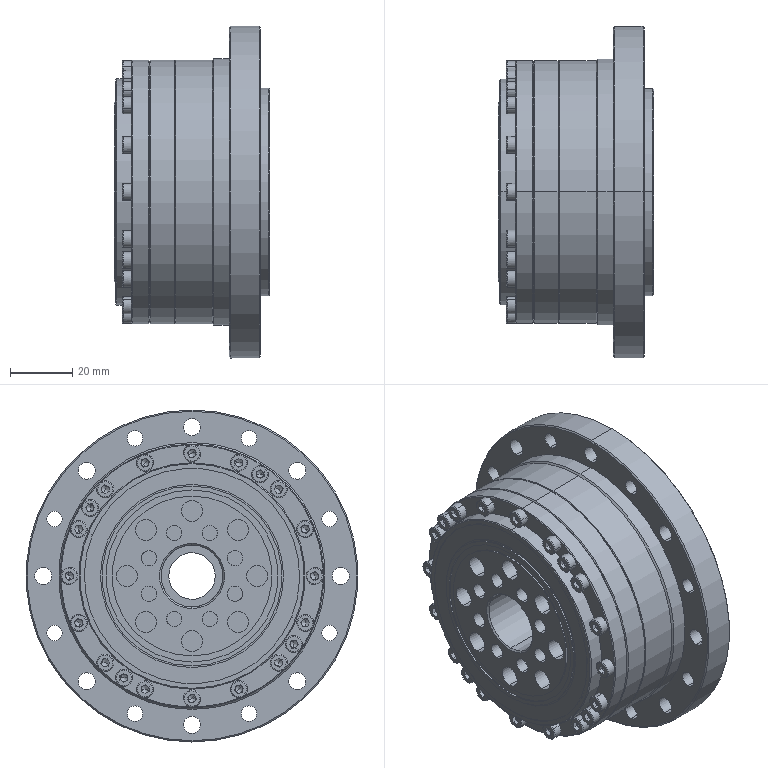Part | SolidWorks | features ICE 1, MBimport 1 | 43 solids | 1161 faces | box 50 x 107 x 107 mm | volume 232615 mm3 | plane 496 | cylinder 302 | cone 159 | torus 112 | sphere 92 | commonest cylinder face diameters 5.5 x64 6.2 x54 5 x32 6 x16 6.8 x16 10 x16